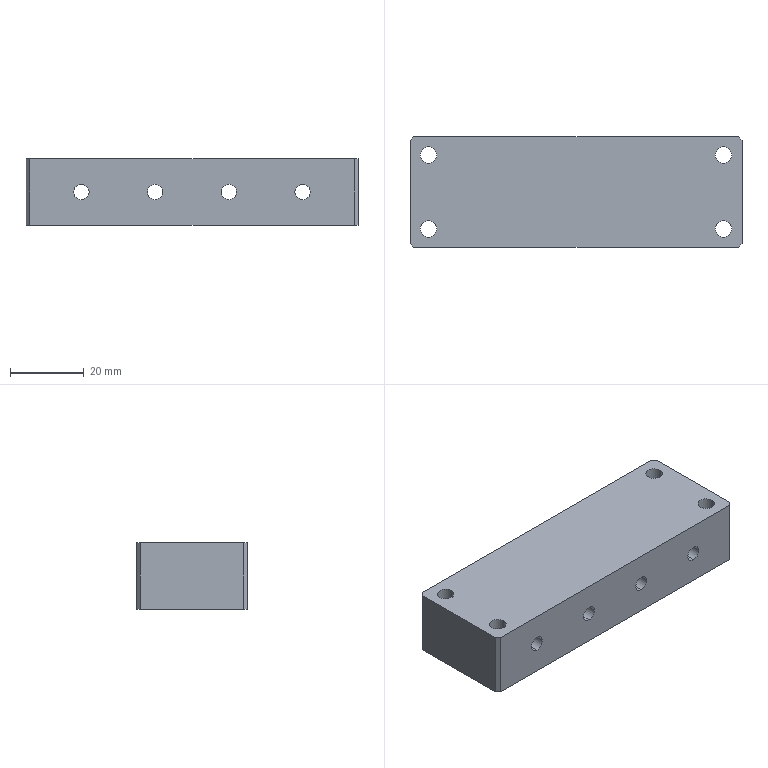Part | SolidWorks | features HoleWzd 3, Chamfer 1, Extrusion 1 | 1 solid | 53 faces | box 90 x 30 x 18 mm | volume 41486 mm3 | cylinder 34 | plane 15 | cone 4 | commonest cylinder face diameters 4.2 x16 4.5 x8 8 x8 7.9 x2